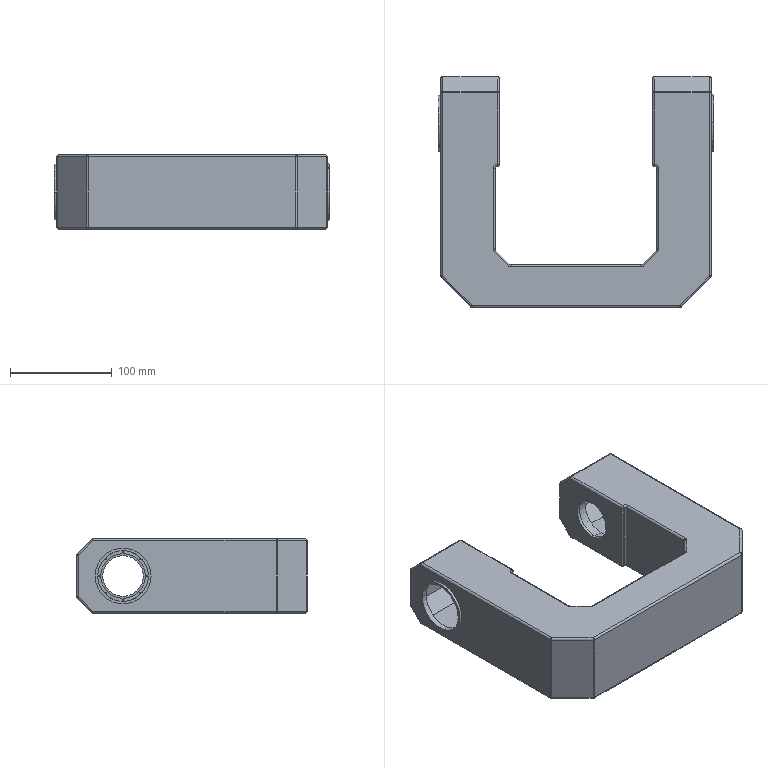Part | SolidWorks | features SavedExtBody 1 | 1 solid | 220 faces | box 271.015 x 226.948 x 73 mm | volume 430356 mm3 | cylinder 112 | plane 66 | sphere 28 | torus 14 | commonest cylinder face diameters 4 x60 1 x32 50 x8 40 x4 44 x4 55 x4